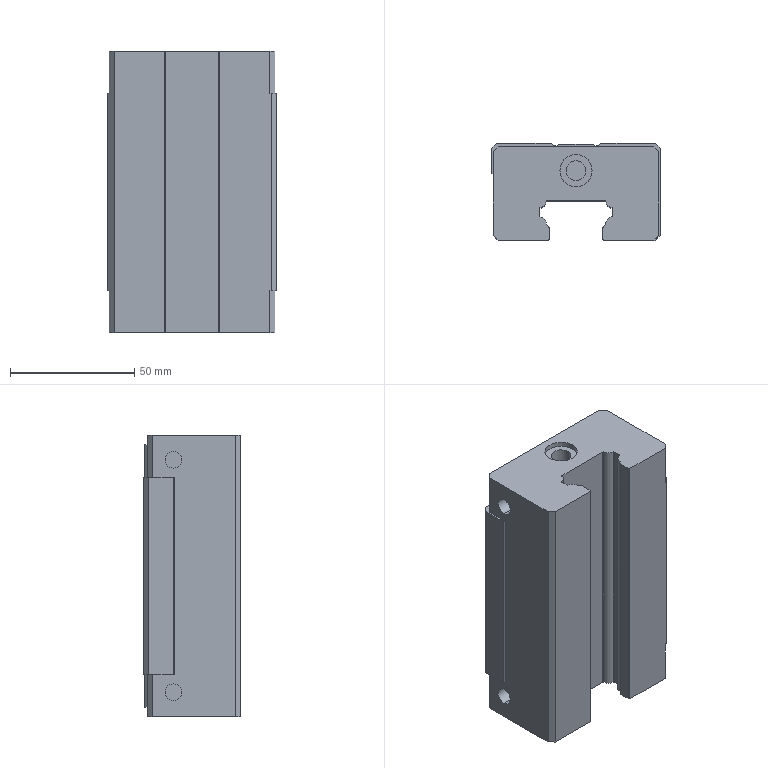Part | SolidWorks | features BaseBody 1 | 1 solid | 115 faces | box 68 x 39 x 113.6 mm | volume 243062 mm3 | plane 66 | cylinder 49 | commonest cylinder face diameters 8 x12 0.92 x8 6.7 x8 6 x5 1.48 x4 2 x4